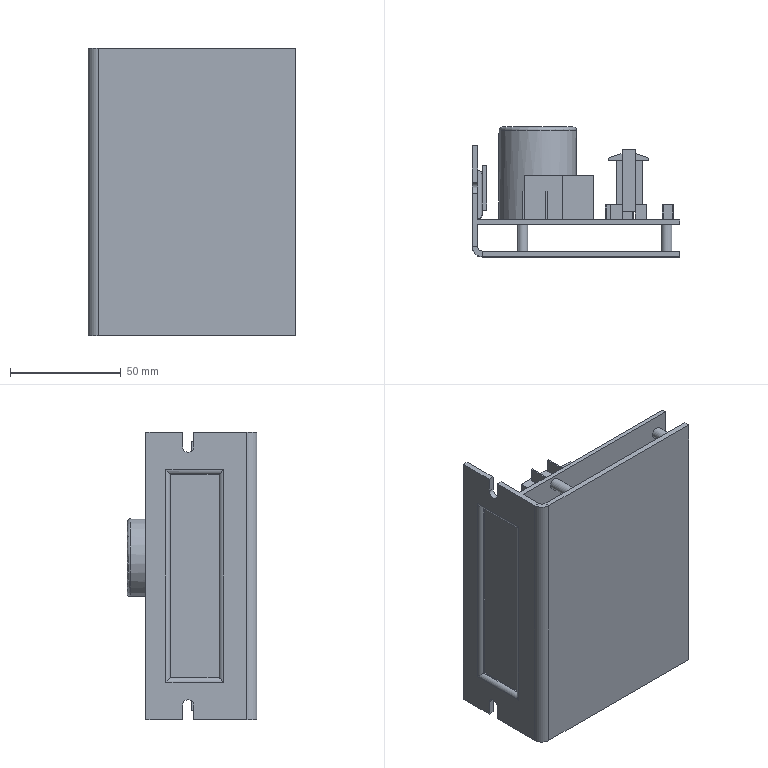Part | STEP file | 509K1002 | 2 solids | 188 faces | box 93.5 x 58.5 x 129.5 mm | volume 128937 mm3 | plane 170 | cylinder 17 | torus 1 | commonest cylinder face diameters 4 x9 5 x6 9 x1 35 x1